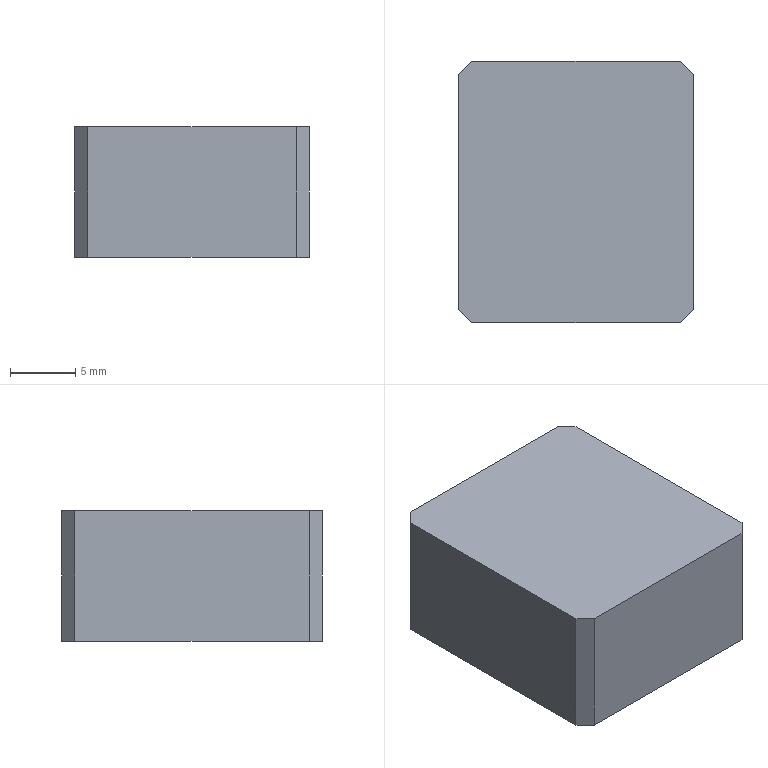Part | STEP file | 2012-06-08-017 | 1 solid | 10 faces | box 18 x 20 x 10 mm | volume 3580 mm3 | plane 10
STEP:
#1=CARTESIAN_POINT('',(0.,0.,0.));
#2=DIRECTION('',(0.,0.,1.));
#3=DIRECTION('',(1.,0.,0.));
#4=AXIS2_PLACEMENT_3D('',#1,#2,#3);
#5=CARTESIAN_POINT('',(9.,-9.,0.));
#6=VERTEX_POINT('',#5);
#7=CARTESIAN_POINT('',(9.,9.,0.));
#8=VERTEX_POINT('',#7);
#9=CARTESIAN_POINT('',(9.,10.,0.));
#10=DIRECTION('',(0.,1.,0.));
#11=VECTOR('',#10,1.);
#12=LINE('',#9,#11);
#13=CARTESIAN_POINT('',(9.,10.,10.));
#14=DIRECTION('',(-1.,0.,0.));
#15=DIRECTION('',(0.,0.,1.));
#16=AXIS2_PLACEMENT_3D('',#13,#14,#15);
#17=PLANE('',#16);
#18=CARTESIAN_POINT('',(-10.,0.));
#19=DIRECTION('',(0.,1.));
#20=VECTOR('',#19,1.);
#21=LINE('',#18,#20);
#22=(GEOMETRIC_REPRESENTATION_CONTEXT(2)PARAMETRIC_REPRESENTATION_CONTEXT()REPRESENTATION_CONTEXT('',''));
#23=DEFINITIONAL_REPRESENTATION('',(#21),#22);
#24=PCURVE('',#17,#23);
#25=CARTESIAN_POINT('',(9.,-10.,0.));
#26=DIRECTION('',(0.,0.,1.));
#27=DIRECTION('',(1.,0.,0.));
#28=AXIS2_PLACEMENT_3D('',#25,#26,#27);
#29=PLANE('',#28);
#30=CARTESIAN_POINT('',(0.,20.));
#31=DIRECTION('',(0.,1.));
#32=VECTOR('',#31,1.);
#33=LINE('',#30,#32);
#34=(GEOMETRIC_REPRESENTATION_CONTEXT(2)PARAMETRIC_REPRESENTATION_CONTEXT()REPRESENTATION_CONTEXT('',''));
#35=DEFINITIONAL_REPRESENTATION('',(#33),#34);
#36=PCURVE('',#29,#35);
#37=SURFACE_CURVE('',#12,(#24,#36),.PCURVE_S1.);
#38=EDGE_CURVE('',#6,#8,#37,.T.);
#39=ORIENTED_EDGE('',*,*,#38,.T.);
#40=CARTESIAN_POINT('',(9.,9.,10.));
#41=VERTEX_POINT('',#40);
#42=CARTESIAN_POINT('',(9.,9.,10.));
#43=DIRECTION('',(0.,0.,1.));
#44=VECTOR('',#43,1.);
#45=LINE('',#42,#44);
#46=CARTESIAN_POINT('',(0.,-1.));
#47=DIRECTION('',(1.,0.));
#48=VECTOR('',#47,1.);
#49=LINE('',#46,#48);
#50=(GEOMETRIC_REPRESENTATION_CONTEXT(2)PARAMETRIC_REPRESENTATION_CONTEXT()REPRESENTATION_CONTEXT('',''));
#51=DEFINITIONAL_REPRESENTATION('',(#49),#50);
#52=PCURVE('',#17,#51);
#53=CARTESIAN_POINT('',(8.,10.,10.));
#54=DIRECTION('',(-0.7071,-0.7071,0.));
#55=DIRECTION('',(0.7071,-0.7071,0.));
#56=AXIS2_PLACEMENT_3D('',#53,#54,#55);
#57=PLANE('',#56);
#58=CARTESIAN_POINT('',(1.414,0.));
#59=DIRECTION('',(0.,1.));
#60=VECTOR('',#59,1.);
#61=LINE('',#58,#60);
#62=(GEOMETRIC_REPRESENTATION_CONTEXT(2)PARAMETRIC_REPRESENTATION_CONTEXT()REPRESENTATION_CONTEXT('',''));
#63=DEFINITIONAL_REPRESENTATION('',(#61),#62);
#64=PCURVE('',#57,#63);
#65=SURFACE_CURVE('',#45,(#52,#64),.PCURVE_S1.);
#66=EDGE_CURVE('',#8,#41,#65,.T.);
#67=ORIENTED_EDGE('',*,*,#66,.T.);
#68=CARTESIAN_POINT('',(9.,-9.,10.));
#69=VERTEX_POINT('',#68);
#70=CARTESIAN_POINT('',(9.,10.,10.));
#71=DIRECTION('',(0.,1.,0.));
#72=VECTOR('',#71,1.);
#73=LINE('',#70,#72);
#74=CARTESIAN_POINT('',(0.,0.));
#75=DIRECTION('',(0.,1.));
#76=VECTOR('',#75,1.);
#77=LINE('',#74,#76);
#78=(GEOMETRIC_REPRESENTATION_CONTEXT(2)PARAMETRIC_REPRESENTATION_CONTEXT()REPRESENTATION_CONTEXT('',''));
#79=DEFINITIONAL_REPRESENTATION('',(#77),#78);
#80=PCURVE('',#17,#79);
#81=CARTESIAN_POINT('',(9.,-10.,10.));
#82=DIRECTION('',(0.,0.,1.));
#83=DIRECTION('',(1.,0.,0.));
#84=AXIS2_PLACEMENT_3D('',#81,#82,#83);
#85=PLANE('',#84);
#86=CARTESIAN_POINT('',(0.,20.));
#87=DIRECTION('',(0.,1.));
#88=VECTOR('',#87,1.);
#89=LINE('',#86,#88);
#90=(GEOMETRIC_REPRESENTATION_CONTEXT(2)PARAMETRIC_REPRESENTATION_CONTEXT()REPRESENTATION_CONTEXT('',''));
#91=DEFINITIONAL_REPRESENTATION('',(#89),#90);
#92=PCURVE('',#85,#91);
#93=SURFACE_CURVE('',#73,(#80,#92),.PCURVE_S1.);
#94=EDGE_CURVE('',#69,#41,#93,.T.);
#95=ORIENTED_EDGE('',*,*,#94,.F.);
#96=CARTESIAN_POINT('',(9.,-9.,10.));
#97=DIRECTION('',(0.,0.,-1.));
#98=VECTOR('',#97,1.);
#99=LINE('',#96,#98);
#100=CARTESIAN_POINT('',(0.,-19.));
#101=DIRECTION('',(-1.,0.));
#102=VECTOR('',#101,1.);
#103=LINE('',#100,#102);
#104=(GEOMETRIC_REPRESENTATION_CONTEXT(2)PARAMETRIC_REPRESENTATION_CONTEXT()REPRESENTATION_CONTEXT('',''));
#105=DEFINITIONAL_REPRESENTATION('',(#103),#104);
#106=PCURVE('',#17,#105);
#107=CARTESIAN_POINT('',(9.,-9.,10.));
#108=DIRECTION('',(-0.7071,0.7071,0.));
#109=DIRECTION('',(-0.7071,-0.7071,0.));
#110=AXIS2_PLACEMENT_3D('',#107,#108,#109);
#111=PLANE('',#110);
#112=CARTESIAN_POINT('',(0.,0.));
#113=DIRECTION('',(0.,-1.));
#114=VECTOR('',#113,1.);
#115=LINE('',#112,#114);
#116=(GEOMETRIC_REPRESENTATION_CONTEXT(2)PARAMETRIC_REPRESENTATION_CONTEXT()REPRESENTATION_CONTEXT('',''));
#117=DEFINITIONAL_REPRESENTATION('',(#115),#116);
#118=PCURVE('',#111,#117);
#119=SURFACE_CURVE('',#99,(#106,#118),.PCURVE_S1.);
#120=EDGE_CURVE('',#69,#6,#119,.T.);
#121=ORIENTED_EDGE('',*,*,#120,.T.);
#122=EDGE_LOOP('',(#39,#67,#95,#121));
#123=FACE_BOUND('',#122,.T.);
#124=ADVANCED_FACE('',(#123),#17,.F.);
#125=CARTESIAN_POINT('',(8.,10.,10.));
#126=VERTEX_POINT('',#125);
#127=CARTESIAN_POINT('',(-8.,10.,10.));
#128=VERTEX_POINT('',#127);
#129=CARTESIAN_POINT('',(-9.,10.,10.));
#130=DIRECTION('',(-1.,0.,0.));
#131=VECTOR('',#130,1.);
#132=LINE('',#129,#131);
#133=CARTESIAN_POINT('',(-9.,10.,10.));
#134=DIRECTION('',(0.,-1.,0.));
#135=DIRECTION('',(0.,0.,-1.));
#136=AXIS2_PLACEMENT_3D('',#133,#134,#135);
#137=PLANE('',#136);
#138=CARTESIAN_POINT('',(0.,0.));
#139=DIRECTION('',(0.,-1.));
#140=VECTOR('',#139,1.);
#141=LINE('',#138,#140);
#142=(GEOMETRIC_REPRESENTATION_CONTEXT(2)PARAMETRIC_REPRESENTATION_CONTEXT()REPRESENTATION_CONTEXT('',''));
#143=DEFINITIONAL_REPRESENTATION('',(#141),#142);
#144=PCURVE('',#137,#143);
#145=CARTESIAN_POINT('',(-18.,20.));
#146=DIRECTION('',(-1.,0.));
#147=VECTOR('',#146,1.);
#148=LINE('',#145,#147);
#149=(GEOMETRIC_REPRESENTATION_CONTEXT(2)PARAMETRIC_REPRESENTATION_CONTEXT()REPRESENTATION_CONTEXT('',''));
#150=DEFINITIONAL_REPRESENTATION('',(#148),#149);
#151=PCURVE('',#85,#150);
#152=SURFACE_CURVE('',#132,(#144,#151),.PCURVE_S1.);
#153=EDGE_CURVE('',#126,#128,#152,.T.);
#154=ORIENTED_EDGE('',*,*,#153,.F.);
#155=CARTESIAN_POINT('',(8.,10.,0.));
#156=VERTEX_POINT('',#155);
#157=CARTESIAN_POINT('',(8.,10.,10.));
#158=DIRECTION('',(0.,0.,-1.));
#159=VECTOR('',#158,1.);
#160=LINE('',#157,#159);
#161=CARTESIAN_POINT('',(0.,17.));
#162=DIRECTION('',(1.,0.));
#163=VECTOR('',#162,1.);
#164=LINE('',#161,#163);
#165=(GEOMETRIC_REPRESENTATION_CONTEXT(2)PARAMETRIC_REPRESENTATION_CONTEXT()REPRESENTATION_CONTEXT('',''));
#166=DEFINITIONAL_REPRESENTATION('',(#164),#165);
#167=PCURVE('',#137,#166);
#168=CARTESIAN_POINT('',(0.,0.));
#169=DIRECTION('',(0.,-1.));
#170=VECTOR('',#169,1.);
#171=LINE('',#168,#170);
#172=(GEOMETRIC_REPRESENTATION_CONTEXT(2)PARAMETRIC_REPRESENTATION_CONTEXT()REPRESENTATION_CONTEXT('',''));
#173=DEFINITIONAL_REPRESENTATION('',(#171),#172);
#174=PCURVE('',#57,#173);
#175=SURFACE_CURVE('',#160,(#167,#174),.PCURVE_S1.);
#176=EDGE_CURVE('',#126,#156,#175,.T.);
#177=ORIENTED_EDGE('',*,*,#176,.T.);
#178=CARTESIAN_POINT('',(-8.,10.,0.));
#179=VERTEX_POINT('',#178);
#180=CARTESIAN_POINT('',(-9.,10.,0.));
#181=DIRECTION('',(-1.,0.,0.));
#182=VECTOR('',#181,1.);
#183=LINE('',#180,#182);
#184=CARTESIAN_POINT('',(10.,0.));
#185=DIRECTION('',(0.,-1.));
#186=VECTOR('',#185,1.);
#187=LINE('',#184,#186);
#188=(GEOMETRIC_REPRESENTATION_CONTEXT(2)PARAMETRIC_REPRESENTATION_CONTEXT()REPRESENTATION_CONTEXT('',''));
#189=DEFINITIONAL_REPRESENTATION('',(#187),#188);
#190=PCURVE('',#137,#189);
#191=CARTESIAN_POINT('',(-18.,20.));
#192=DIRECTION('',(-1.,0.));
#193=VECTOR('',#192,1.);
#194=LINE('',#191,#193);
#195=(GEOMETRIC_REPRESENTATION_CONTEXT(2)PARAMETRIC_REPRESENTATION_CONTEXT()REPRESENTATION_CONTEXT('',''));
#196=DEFINITIONAL_REPRESENTATION('',(#194),#195);
#197=PCURVE('',#29,#196);
#198=SURFACE_CURVE('',#183,(#190,#197),.PCURVE_S1.);
#199=EDGE_CURVE('',#156,#179,#198,.T.);
#200=ORIENTED_EDGE('',*,*,#199,.T.);
#201=CARTESIAN_POINT('',(-8.,10.,10.));
#202=DIRECTION('',(0.,0.,1.));
#203=VECTOR('',#202,1.);
#204=LINE('',#201,#203);
#205=CARTESIAN_POINT('',(0.,1.));
#206=DIRECTION('',(-1.,0.));
#207=VECTOR('',#206,1.);
#208=LINE('',#205,#207);
#209=(GEOMETRIC_REPRESENTATION_CONTEXT(2)PARAMETRIC_REPRESENTATION_CONTEXT()REPRESENTATION_CONTEXT('',''));
#210=DEFINITIONAL_REPRESENTATION('',(#208),#209);
#211=PCURVE('',#137,#210);
#212=CARTESIAN_POINT('',(-9.,9.,10.));
#213=DIRECTION('',(0.7071,-0.7071,0.));
#214=DIRECTION('',(0.7071,0.7071,0.));
#215=AXIS2_PLACEMENT_3D('',#212,#213,#214);
#216=PLANE('',#215);
#217=CARTESIAN_POINT('',(1.414,0.));
#218=DIRECTION('',(0.,1.));
#219=VECTOR('',#218,1.);
#220=LINE('',#217,#219);
#221=(GEOMETRIC_REPRESENTATION_CONTEXT(2)PARAMETRIC_REPRESENTATION_CONTEXT()REPRESENTATION_CONTEXT('',''));
#222=DEFINITIONAL_REPRESENTATION('',(#220),#221);
#223=PCURVE('',#216,#222);
#224=SURFACE_CURVE('',#204,(#211,#223),.PCURVE_S1.);
#225=EDGE_CURVE('',#179,#128,#224,.T.);
#226=ORIENTED_EDGE('',*,*,#225,.T.);
#227=EDGE_LOOP('',(#154,#177,#200,#226));
#228=FACE_BOUND('',#227,.T.);
#229=ADVANCED_FACE('',(#228),#137,.F.);
#230=CARTESIAN_POINT('',(-9.,9.,10.));
#231=VERTEX_POINT('',#230);
#232=CARTESIAN_POINT('',(-9.,-9.,10.));
#233=VERTEX_POINT('',#232);
#234=CARTESIAN_POINT('',(-9.,10.,10.));
#235=DIRECTION('',(0.,-1.,0.));
#236=VECTOR('',#235,1.);
#237=LINE('',#234,#236);
#238=CARTESIAN_POINT('',(-9.,10.,10.));
#239=DIRECTION('',(1.,0.,0.));
#240=DIRECTION('',(0.,1.,0.));
#241=AXIS2_PLACEMENT_3D('',#238,#239,#240);
#242=PLANE('',#241);
#243=CARTESIAN_POINT('',(0.,0.));
#244=DIRECTION('',(-1.,0.));
#245=VECTOR('',#244,1.);
#246=LINE('',#243,#245);
#247=(GEOMETRIC_REPRESENTATION_CONTEXT(2)PARAMETRIC_REPRESENTATION_CONTEXT()REPRESENTATION_CONTEXT('',''));
#248=DEFINITIONAL_REPRESENTATION('',(#246),#247);
#249=PCURVE('',#242,#248);
#250=CARTESIAN_POINT('',(-18.,20.));
#251=DIRECTION('',(0.,-1.));
#252=VECTOR('',#251,1.);
#253=LINE('',#250,#252);
#254=(GEOMETRIC_REPRESENTATION_CONTEXT(2)PARAMETRIC_REPRESENTATION_CONTEXT()REPRESENTATION_CONTEXT('',''));
#255=DEFINITIONAL_REPRESENTATION('',(#253),#254);
#256=PCURVE('',#85,#255);
#257=SURFACE_CURVE('',#237,(#249,#256),.PCURVE_S1.);
#258=EDGE_CURVE('',#231,#233,#257,.T.);
#259=ORIENTED_EDGE('',*,*,#258,.F.);
#260=CARTESIAN_POINT('',(-9.,9.,0.));
#261=VERTEX_POINT('',#260);
#262=CARTESIAN_POINT('',(-9.,9.,10.));
#263=DIRECTION('',(0.,0.,-1.));
#264=VECTOR('',#263,1.);
#265=LINE('',#262,#264);
#266=CARTESIAN_POINT('',(-1.,0.));
#267=DIRECTION('',(0.,-1.));
#268=VECTOR('',#267,1.);
#269=LINE('',#266,#268);
#270=(GEOMETRIC_REPRESENTATION_CONTEXT(2)PARAMETRIC_REPRESENTATION_CONTEXT()REPRESENTATION_CONTEXT('',''));
#271=DEFINITIONAL_REPRESENTATION('',(#269),#270);
#272=PCURVE('',#242,#271);
#273=CARTESIAN_POINT('',(0.,0.));
#274=DIRECTION('',(0.,-1.));
#275=VECTOR('',#274,1.);
#276=LINE('',#273,#275);
#277=(GEOMETRIC_REPRESENTATION_CONTEXT(2)PARAMETRIC_REPRESENTATION_CONTEXT()REPRESENTATION_CONTEXT('',''));
#278=DEFINITIONAL_REPRESENTATION('',(#276),#277);
#279=PCURVE('',#216,#278);
#280=SURFACE_CURVE('',#265,(#272,#279),.PCURVE_S1.);
#281=EDGE_CURVE('',#231,#261,#280,.T.);
#282=ORIENTED_EDGE('',*,*,#281,.T.);
#283=CARTESIAN_POINT('',(-9.,-9.,0.));
#284=VERTEX_POINT('',#283);
#285=CARTESIAN_POINT('',(-9.,10.,0.));
#286=DIRECTION('',(0.,-1.,0.));
#287=VECTOR('',#286,1.);
#288=LINE('',#285,#287);
#289=CARTESIAN_POINT('',(0.,-10.));
#290=DIRECTION('',(-1.,0.));
#291=VECTOR('',#290,1.);
#292=LINE('',#289,#291);
#293=(GEOMETRIC_REPRESENTATION_CONTEXT(2)PARAMETRIC_REPRESENTATION_CONTEXT()REPRESENTATION_CONTEXT('',''));
#294=DEFINITIONAL_REPRESENTATION('',(#292),#293);
#295=PCURVE('',#242,#294);
#296=CARTESIAN_POINT('',(-18.,20.));
#297=DIRECTION('',(0.,-1.));
#298=VECTOR('',#297,1.);
#299=LINE('',#296,#298);
#300=(GEOMETRIC_REPRESENTATION_CONTEXT(2)PARAMETRIC_REPRESENTATION_CONTEXT()REPRESENTATION_CONTEXT('',''));
#301=DEFINITIONAL_REPRESENTATION('',(#299),#300);
#302=PCURVE('',#29,#301);
#303=SURFACE_CURVE('',#288,(#295,#302),.PCURVE_S1.);
#304=EDGE_CURVE('',#261,#284,#303,.T.);
#305=ORIENTED_EDGE('',*,*,#304,.T.);
#306=CARTESIAN_POINT('',(-9.,-9.,10.));
#307=DIRECTION('',(0.,0.,1.));
#308=VECTOR('',#307,1.);
#309=LINE('',#306,#308);
#310=CARTESIAN_POINT('',(-19.,0.));
#311=DIRECTION('',(0.,1.));
#312=VECTOR('',#311,1.);
#313=LINE('',#310,#312);
#314=(GEOMETRIC_REPRESENTATION_CONTEXT(2)PARAMETRIC_REPRESENTATION_CONTEXT()REPRESENTATION_CONTEXT('',''));
#315=DEFINITIONAL_REPRESENTATION('',(#313),#314);
#316=PCURVE('',#242,#315);
#317=CARTESIAN_POINT('',(-8.,-10.,10.));
#318=DIRECTION('',(0.7071,0.7071,0.));
#319=DIRECTION('',(-0.7071,0.7071,0.));
#320=AXIS2_PLACEMENT_3D('',#317,#318,#319);
#321=PLANE('',#320);
#322=CARTESIAN_POINT('',(1.414,0.));
#323=DIRECTION('',(0.,1.));
#324=VECTOR('',#323,1.);
#325=LINE('',#322,#324);
#326=(GEOMETRIC_REPRESENTATION_CONTEXT(2)PARAMETRIC_REPRESENTATION_CONTEXT()REPRESENTATION_CONTEXT('',''));
#327=DEFINITIONAL_REPRESENTATION('',(#325),#326);
#328=PCURVE('',#321,#327);
#329=SURFACE_CURVE('',#309,(#316,#328),.PCURVE_S1.);
#330=EDGE_CURVE('',#284,#233,#329,.T.);
#331=ORIENTED_EDGE('',*,*,#330,.T.);
#332=EDGE_LOOP('',(#259,#282,#305,#331));
#333=FACE_BOUND('',#332,.T.);
#334=ADVANCED_FACE('',(#333),#242,.F.);
#335=CARTESIAN_POINT('',(-8.,-10.,0.));
#336=VERTEX_POINT('',#335);
#337=CARTESIAN_POINT('',(8.,-10.,0.));
#338=VERTEX_POINT('',#337);
#339=CARTESIAN_POINT('',(-9.,-10.,0.));
#340=DIRECTION('',(1.,0.,0.));
#341=VECTOR('',#340,1.);
#342=LINE('',#339,#341);
#343=CARTESIAN_POINT('',(-9.,-10.,10.));
#344=DIRECTION('',(0.,1.,0.));
#345=DIRECTION('',(0.,0.,1.));
#346=AXIS2_PLACEMENT_3D('',#343,#344,#345);
#347=PLANE('',#346);
#348=CARTESIAN_POINT('',(-10.,0.));
#349=DIRECTION('',(0.,1.));
#350=VECTOR('',#349,1.);
#351=LINE('',#348,#350);
#352=(GEOMETRIC_REPRESENTATION_CONTEXT(2)PARAMETRIC_REPRESENTATION_CONTEXT()REPRESENTATION_CONTEXT('',''));
#353=DEFINITIONAL_REPRESENTATION('',(#351),#352);
#354=PCURVE('',#347,#353);
#355=CARTESIAN_POINT('',(-18.,0.));
#356=DIRECTION('',(1.,0.));
#357=VECTOR('',#356,1.);
#358=LINE('',#355,#357);
#359=(GEOMETRIC_REPRESENTATION_CONTEXT(2)PARAMETRIC_REPRESENTATION_CONTEXT()REPRESENTATION_CONTEXT('',''));
#360=DEFINITIONAL_REPRESENTATION('',(#358),#359);
#361=PCURVE('',#29,#360);
#362=SURFACE_CURVE('',#342,(#354,#361),.PCURVE_S1.);
#363=EDGE_CURVE('',#336,#338,#362,.T.);
#364=ORIENTED_EDGE('',*,*,#363,.T.);
#365=CARTESIAN_POINT('',(8.,-10.,10.));
#366=VERTEX_POINT('',#365);
#367=CARTESIAN_POINT('',(8.,-10.,10.));
#368=DIRECTION('',(0.,0.,1.));
#369=VECTOR('',#368,1.);
#370=LINE('',#367,#369);
#371=CARTESIAN_POINT('',(0.,17.));
#372=DIRECTION('',(1.,0.));
#373=VECTOR('',#372,1.);
#374=LINE('',#371,#373);
#375=(GEOMETRIC_REPRESENTATION_CONTEXT(2)PARAMETRIC_REPRESENTATION_CONTEXT()REPRESENTATION_CONTEXT('',''));
#376=DEFINITIONAL_REPRESENTATION('',(#374),#375);
#377=PCURVE('',#347,#376);
#378=CARTESIAN_POINT('',(1.414,0.));
#379=DIRECTION('',(0.,1.));
#380=VECTOR('',#379,1.);
#381=LINE('',#378,#380);
#382=(GEOMETRIC_REPRESENTATION_CONTEXT(2)PARAMETRIC_REPRESENTATION_CONTEXT()REPRESENTATION_CONTEXT('',''));
#383=DEFINITIONAL_REPRESENTATION('',(#381),#382);
#384=PCURVE('',#111,#383);
#385=SURFACE_CURVE('',#370,(#377,#384),.PCURVE_S1.);
#386=EDGE_CURVE('',#338,#366,#385,.T.);
#387=ORIENTED_EDGE('',*,*,#386,.T.);
#388=CARTESIAN_POINT('',(-8.,-10.,10.));
#389=VERTEX_POINT('',#388);
#390=CARTESIAN_POINT('',(-9.,-10.,10.));
#391=DIRECTION('',(1.,0.,0.));
#392=VECTOR('',#391,1.);
#393=LINE('',#390,#392);
#394=CARTESIAN_POINT('',(0.,0.));
#395=DIRECTION('',(0.,1.));
#396=VECTOR('',#395,1.);
#397=LINE('',#394,#396);
#398=(GEOMETRIC_REPRESENTATION_CONTEXT(2)PARAMETRIC_REPRESENTATION_CONTEXT()REPRESENTATION_CONTEXT('',''));
#399=DEFINITIONAL_REPRESENTATION('',(#397),#398);
#400=PCURVE('',#347,#399);
#401=CARTESIAN_POINT('',(-18.,0.));
#402=DIRECTION('',(1.,0.));
#403=VECTOR('',#402,1.);
#404=LINE('',#401,#403);
#405=(GEOMETRIC_REPRESENTATION_CONTEXT(2)PARAMETRIC_REPRESENTATION_CONTEXT()REPRESENTATION_CONTEXT('',''));
#406=DEFINITIONAL_REPRESENTATION('',(#404),#405);
#407=PCURVE('',#85,#406);
#408=SURFACE_CURVE('',#393,(#400,#407),.PCURVE_S1.);
#409=EDGE_CURVE('',#389,#366,#408,.T.);
#410=ORIENTED_EDGE('',*,*,#409,.F.);
#411=CARTESIAN_POINT('',(-8.,-10.,10.));
#412=DIRECTION('',(0.,0.,-1.));
#413=VECTOR('',#412,1.);
#414=LINE('',#411,#413);
#415=CARTESIAN_POINT('',(0.,1.));
#416=DIRECTION('',(-1.,0.));
#417=VECTOR('',#416,1.);
#418=LINE('',#415,#417);
#419=(GEOMETRIC_REPRESENTATION_CONTEXT(2)PARAMETRIC_REPRESENTATION_CONTEXT()REPRESENTATION_CONTEXT('',''));
#420=DEFINITIONAL_REPRESENTATION('',(#418),#419);
#421=PCURVE('',#347,#420);
#422=CARTESIAN_POINT('',(0.,0.));
#423=DIRECTION('',(0.,-1.));
#424=VECTOR('',#423,1.);
#425=LINE('',#422,#424);
#426=(GEOMETRIC_REPRESENTATION_CONTEXT(2)PARAMETRIC_REPRESENTATION_CONTEXT()REPRESENTATION_CONTEXT('',''));
#427=DEFINITIONAL_REPRESENTATION('',(#425),#426);
#428=PCURVE('',#321,#427);
#429=SURFACE_CURVE('',#414,(#421,#428),.PCURVE_S1.);
#430=EDGE_CURVE('',#389,#336,#429,.T.);
#431=ORIENTED_EDGE('',*,*,#430,.T.);
#432=EDGE_LOOP('',(#364,#387,#410,#431));
#433=FACE_BOUND('',#432,.T.);
#434=ADVANCED_FACE('',(#433),#347,.F.);
#435=ORIENTED_EDGE('',*,*,#94,.T.);
#436=CARTESIAN_POINT('',(18.5,-0.5,10.));
#437=DIRECTION('',(-0.7071,0.7071,0.));
#438=VECTOR('',#437,1.);
#439=LINE('',#436,#438);
#440=CARTESIAN_POINT('',(9.5,9.5));
#441=DIRECTION('',(-0.7071,0.7071));
#442=VECTOR('',#441,1.);
#443=LINE('',#440,#442);
#444=(GEOMETRIC_REPRESENTATION_CONTEXT(2)PARAMETRIC_REPRESENTATION_CONTEXT()REPRESENTATION_CONTEXT('',''));
#445=DEFINITIONAL_REPRESENTATION('',(#443),#444);
#446=PCURVE('',#85,#445);
#447=CARTESIAN_POINT('',(14.849,0.));
#448=DIRECTION('',(-1.,0.));
#449=VECTOR('',#448,1.);
#450=LINE('',#447,#449);
#451=(GEOMETRIC_REPRESENTATION_CONTEXT(2)PARAMETRIC_REPRESENTATION_CONTEXT()REPRESENTATION_CONTEXT('',''));
#452=DEFINITIONAL_REPRESENTATION('',(#450),#451);
#453=PCURVE('',#57,#452);
#454=SURFACE_CURVE('',#439,(#446,#453),.PCURVE_S1.);
#455=EDGE_CURVE('',#41,#126,#454,.T.);
#456=ORIENTED_EDGE('',*,*,#455,.T.);
#457=ORIENTED_EDGE('',*,*,#153,.T.);
#458=CARTESIAN_POINT('',(-9.5,8.5,10.));
#459=DIRECTION('',(-0.7071,-0.7071,0.));
#460=VECTOR('',#459,1.);
#461=LINE('',#458,#460);
#462=CARTESIAN_POINT('',(-18.5,18.5));
#463=DIRECTION('',(-0.7071,-0.7071));
#464=VECTOR('',#463,1.);
#465=LINE('',#462,#464);
#466=(GEOMETRIC_REPRESENTATION_CONTEXT(2)PARAMETRIC_REPRESENTATION_CONTEXT()REPRESENTATION_CONTEXT('',''));
#467=DEFINITIONAL_REPRESENTATION('',(#465),#466);
#468=PCURVE('',#85,#467);
#469=CARTESIAN_POINT('',(-0.7071,0.));
#470=DIRECTION('',(-1.,0.));
#471=VECTOR('',#470,1.);
#472=LINE('',#469,#471);
#473=(GEOMETRIC_REPRESENTATION_CONTEXT(2)PARAMETRIC_REPRESENTATION_CONTEXT()REPRESENTATION_CONTEXT('',''));
#474=DEFINITIONAL_REPRESENTATION('',(#472),#473);
#475=PCURVE('',#216,#474);
#476=SURFACE_CURVE('',#461,(#468,#475),.PCURVE_S1.);
#477=EDGE_CURVE('',#128,#231,#476,.T.);
#478=ORIENTED_EDGE('',*,*,#477,.T.);
#479=ORIENTED_EDGE('',*,*,#258,.T.);
#480=CARTESIAN_POINT('',(0.5,-18.5,10.));
#481=DIRECTION('',(0.7071,-0.7071,0.));
#482=VECTOR('',#481,1.);
#483=LINE('',#480,#482);
#484=CARTESIAN_POINT('',(-8.5,-8.5));
#485=DIRECTION('',(0.7071,-0.7071));
#486=VECTOR('',#485,1.);
#487=LINE('',#484,#486);
#488=(GEOMETRIC_REPRESENTATION_CONTEXT(2)PARAMETRIC_REPRESENTATION_CONTEXT()REPRESENTATION_CONTEXT('',''));
#489=DEFINITIONAL_REPRESENTATION('',(#487),#488);
#490=PCURVE('',#85,#489);
#491=CARTESIAN_POINT('',(-12.021,0.));
#492=DIRECTION('',(-1.,0.));
#493=VECTOR('',#492,1.);
#494=LINE('',#491,#493);
#495=(GEOMETRIC_REPRESENTATION_CONTEXT(2)PARAMETRIC_REPRESENTATION_CONTEXT()REPRESENTATION_CONTEXT('',''));
#496=DEFINITIONAL_REPRESENTATION('',(#494),#495);
#497=PCURVE('',#321,#496);
#498=SURFACE_CURVE('',#483,(#490,#497),.PCURVE_S1.);
#499=EDGE_CURVE('',#233,#389,#498,.T.);
#500=ORIENTED_EDGE('',*,*,#499,.T.);
#501=ORIENTED_EDGE('',*,*,#409,.T.);
#502=CARTESIAN_POINT('',(8.5,-9.5,10.));
#503=DIRECTION('',(0.7071,0.7071,0.));
#504=VECTOR('',#503,1.);
#505=LINE('',#502,#504);
#506=CARTESIAN_POINT('',(-0.5,0.5));
#507=DIRECTION('',(0.7071,0.7071));
#508=VECTOR('',#507,1.);
#509=LINE('',#506,#508);
#510=(GEOMETRIC_REPRESENTATION_CONTEXT(2)PARAMETRIC_REPRESENTATION_CONTEXT()REPRESENTATION_CONTEXT('',''));
#511=DEFINITIONAL_REPRESENTATION('',(#509),#510);
#512=PCURVE('',#85,#511);
#513=CARTESIAN_POINT('',(0.7071,0.));
#514=DIRECTION('',(-1.,0.));
#515=VECTOR('',#514,1.);
#516=LINE('',#513,#515);
#517=(GEOMETRIC_REPRESENTATION_CONTEXT(2)PARAMETRIC_REPRESENTATION_CONTEXT()REPRESENTATION_CONTEXT('',''));
#518=DEFINITIONAL_REPRESENTATION('',(#516),#517);
#519=PCURVE('',#111,#518);
#520=SURFACE_CURVE('',#505,(#512,#519),.PCURVE_S1.);
#521=EDGE_CURVE('',#366,#69,#520,.T.);
#522=ORIENTED_EDGE('',*,*,#521,.T.);
#523=EDGE_LOOP('',(#435,#456,#457,#478,#479,#500,#501,#522));
#524=FACE_BOUND('',#523,.T.);
#525=ADVANCED_FACE('',(#524),#85,.T.);
#526=ORIENTED_EDGE('',*,*,#199,.F.);
#527=CARTESIAN_POINT('',(8.,10.,0.));
#528=DIRECTION('',(0.7071,-0.7071,0.));
#529=VECTOR('',#528,1.);
#530=LINE('',#527,#529);
#531=CARTESIAN_POINT('',(-1.,20.));
#532=DIRECTION('',(0.7071,-0.7071));
#533=VECTOR('',#532,1.);
#534=LINE('',#531,#533);
#535=(GEOMETRIC_REPRESENTATION_CONTEXT(2)PARAMETRIC_REPRESENTATION_CONTEXT()REPRESENTATION_CONTEXT('',''));
#536=DEFINITIONAL_REPRESENTATION('',(#534),#535);
#537=PCURVE('',#29,#536);
#538=CARTESIAN_POINT('',(0.,-10.));
#539=DIRECTION('',(1.,0.));
#540=VECTOR('',#539,1.);
#541=LINE('',#538,#540);
#542=(GEOMETRIC_REPRESENTATION_CONTEXT(2)PARAMETRIC_REPRESENTATION_CONTEXT()REPRESENTATION_CONTEXT('',''));
#543=DEFINITIONAL_REPRESENTATION('',(#541),#542);
#544=PCURVE('',#57,#543);
#545=SURFACE_CURVE('',#530,(#537,#544),.PCURVE_S1.);
#546=EDGE_CURVE('',#156,#8,#545,.T.);
#547=ORIENTED_EDGE('',*,*,#546,.T.);
#548=ORIENTED_EDGE('',*,*,#38,.F.);
#549=CARTESIAN_POINT('',(9.,-9.,0.));
#550=DIRECTION('',(-0.7071,-0.7071,0.));
#551=VECTOR('',#550,1.);
#552=LINE('',#549,#551);
#553=CARTESIAN_POINT('',(0.,1.));
#554=DIRECTION('',(-0.7071,-0.7071));
#555=VECTOR('',#554,1.);
#556=LINE('',#553,#555);
#557=(GEOMETRIC_REPRESENTATION_CONTEXT(2)PARAMETRIC_REPRESENTATION_CONTEXT()REPRESENTATION_CONTEXT('',''));
#558=DEFINITIONAL_REPRESENTATION('',(#556),#557);
#559=PCURVE('',#29,#558);
#560=CARTESIAN_POINT('',(0.,-10.));
#561=DIRECTION('',(1.,0.));
#562=VECTOR('',#561,1.);
#563=LINE('',#560,#562);
#564=(GEOMETRIC_REPRESENTATION_CONTEXT(2)PARAMETRIC_REPRESENTATION_CONTEXT()REPRESENTATION_CONTEXT('',''));
#565=DEFINITIONAL_REPRESENTATION('',(#563),#564);
#566=PCURVE('',#111,#565);
#567=SURFACE_CURVE('',#552,(#559,#566),.PCURVE_S1.);
#568=EDGE_CURVE('',#6,#338,#567,.T.);
#569=ORIENTED_EDGE('',*,*,#568,.T.);
#570=ORIENTED_EDGE('',*,*,#363,.F.);
#571=CARTESIAN_POINT('',(-8.,-10.,0.));
#572=DIRECTION('',(-0.7071,0.7071,0.));
#573=VECTOR('',#572,1.);
#574=LINE('',#571,#573);
#575=CARTESIAN_POINT('',(-17.,0.));
#576=DIRECTION('',(-0.7071,0.7071));
#577=VECTOR('',#576,1.);
#578=LINE('',#575,#577);
#579=(GEOMETRIC_REPRESENTATION_CONTEXT(2)PARAMETRIC_REPRESENTATION_CONTEXT()REPRESENTATION_CONTEXT('',''));
#580=DEFINITIONAL_REPRESENTATION('',(#578),#579);
#581=PCURVE('',#29,#580);
#582=CARTESIAN_POINT('',(0.,-10.));
#583=DIRECTION('',(1.,0.));
#584=VECTOR('',#583,1.);
#585=LINE('',#582,#584);
#586=(GEOMETRIC_REPRESENTATION_CONTEXT(2)PARAMETRIC_REPRESENTATION_CONTEXT()REPRESENTATION_CONTEXT('',''));
#587=DEFINITIONAL_REPRESENTATION('',(#585),#586);
#588=PCURVE('',#321,#587);
#589=SURFACE_CURVE('',#574,(#581,#588),.PCURVE_S1.);
#590=EDGE_CURVE('',#336,#284,#589,.T.);
#591=ORIENTED_EDGE('',*,*,#590,.T.);
#592=ORIENTED_EDGE('',*,*,#304,.F.);
#593=CARTESIAN_POINT('',(-9.,9.,0.));
#594=DIRECTION('',(0.7071,0.7071,0.));
#595=VECTOR('',#594,1.);
#596=LINE('',#593,#595);
#597=CARTESIAN_POINT('',(-18.,19.));
#598=DIRECTION('',(0.7071,0.7071));
#599=VECTOR('',#598,1.);
#600=LINE('',#597,#599);
#601=(GEOMETRIC_REPRESENTATION_CONTEXT(2)PARAMETRIC_REPRESENTATION_CONTEXT()REPRESENTATION_CONTEXT('',''));
#602=DEFINITIONAL_REPRESENTATION('',(#600),#601);
#603=PCURVE('',#29,#602);
#604=CARTESIAN_POINT('',(0.,-10.));
#605=DIRECTION('',(1.,0.));
#606=VECTOR('',#605,1.);
#607=LINE('',#604,#606);
#608=(GEOMETRIC_REPRESENTATION_CONTEXT(2)PARAMETRIC_REPRESENTATION_CONTEXT()REPRESENTATION_CONTEXT('',''));
#609=DEFINITIONAL_REPRESENTATION('',(#607),#608);
#610=PCURVE('',#216,#609);
#611=SURFACE_CURVE('',#596,(#603,#610),.PCURVE_S1.);
#612=EDGE_CURVE('',#261,#179,#611,.T.);
#613=ORIENTED_EDGE('',*,*,#612,.T.);
#614=EDGE_LOOP('',(#526,#547,#548,#569,#570,#591,#592,#613));
#615=FACE_BOUND('',#614,.T.);
#616=ADVANCED_FACE('',(#615),#29,.F.);
#617=ORIENTED_EDGE('',*,*,#455,.F.);
#618=ORIENTED_EDGE('',*,*,#66,.F.);
#619=ORIENTED_EDGE('',*,*,#546,.F.);
#620=ORIENTED_EDGE('',*,*,#176,.F.);
#621=EDGE_LOOP('',(#617,#618,#619,#620));
#622=FACE_BOUND('',#621,.T.);
#623=ADVANCED_FACE('',(#622),#57,.F.);
#624=ORIENTED_EDGE('',*,*,#521,.F.);
#625=ORIENTED_EDGE('',*,*,#386,.F.);
#626=ORIENTED_EDGE('',*,*,#568,.F.);
#627=ORIENTED_EDGE('',*,*,#120,.F.);
#628=EDGE_LOOP('',(#624,#625,#626,#627));
#629=FACE_BOUND('',#628,.T.);
#630=ADVANCED_FACE('',(#629),#111,.F.);
#631=ORIENTED_EDGE('',*,*,#477,.F.);
#632=ORIENTED_EDGE('',*,*,#225,.F.);
#633=ORIENTED_EDGE('',*,*,#612,.F.);
#634=ORIENTED_EDGE('',*,*,#281,.F.);
#635=EDGE_LOOP('',(#631,#632,#633,#634));
#636=FACE_BOUND('',#635,.T.);
#637=ADVANCED_FACE('',(#636),#216,.F.);
#638=ORIENTED_EDGE('',*,*,#499,.F.);
#639=ORIENTED_EDGE('',*,*,#330,.F.);
#640=ORIENTED_EDGE('',*,*,#590,.F.);
#641=ORIENTED_EDGE('',*,*,#430,.F.);
#642=EDGE_LOOP('',(#638,#639,#640,#641));
#643=FACE_BOUND('',#642,.T.);
#644=ADVANCED_FACE('',(#643),#321,.F.);
#645=CLOSED_SHELL('',(#124,#229,#334,#434,#525,#616,#623,#630,#637,#644));
#646=MANIFOLD_SOLID_BREP('',#645);
#647=(LENGTH_UNIT()NAMED_UNIT(*)SI_UNIT(.MILLI.,.METRE.));
#648=UNCERTAINTY_MEASURE_WITH_UNIT(LENGTH_MEASURE(0.0000001),#647,'','');
#649=(NAMED_UNIT(*)PLANE_ANGLE_UNIT()SI_UNIT($,.RADIAN.));
#650=(NAMED_UNIT(*)SI_UNIT($,.STERADIAN.)SOLID_ANGLE_UNIT());
#651=(GEOMETRIC_REPRESENTATION_CONTEXT(3)GLOBAL_UNCERTAINTY_ASSIGNED_CONTEXT((#648))GLOBAL_UNIT_ASSIGNED_CONTEXT((#647,#649,#650))REPRESENTATION_CONTEXT('',''));
#652=ADVANCED_BREP_SHAPE_REPRESENTATION('',(#4,#646),#651);